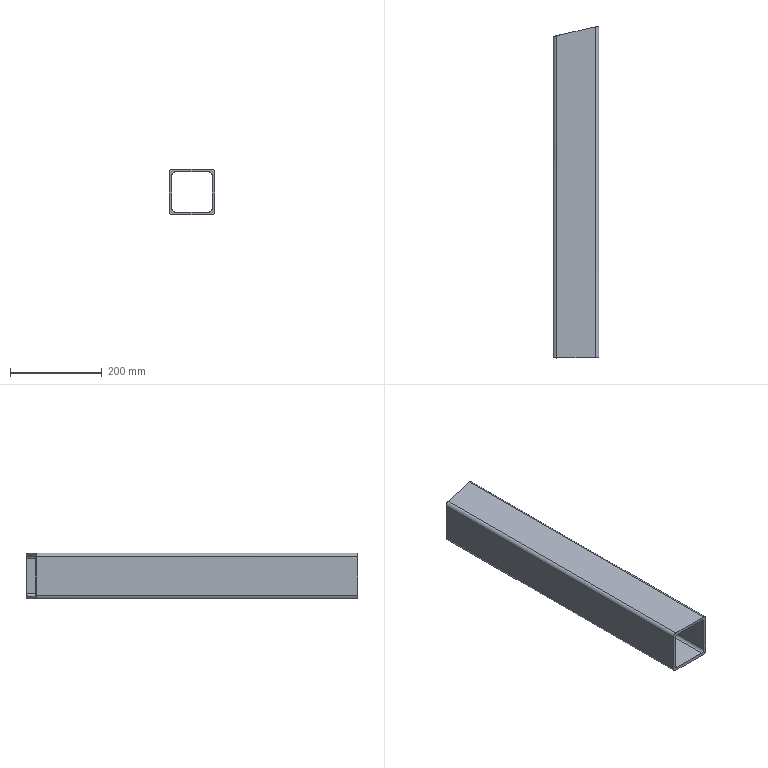Part | SolidWorks | features Extrusion 1, ICE 1 | 1 solid | 18 faces | box 100 x 723 x 100 mm | volume 1666387 mm3 | plane 10 | cylinder 8 | commonest cylinder face diameters 12.6 x4 15.75 x4
STEP:
#1=CARTESIAN_POINT('',(100.,-361.5,-90.6));
#2=VERTEX_POINT('',#1);
#3=CARTESIAN_POINT('',(92.125,-361.5,-98.475));
#4=VERTEX_POINT('',#3);
#5=CARTESIAN_POINT('',(92.125,-361.5,-90.6));
#6=DIRECTION('',(0.,1.,0.));
#7=DIRECTION('',(0.,0.,1.));
#8=AXIS2_PLACEMENT_3D('',#5,#6,#7);
#9=CIRCLE('',#8,7.875);
#10=EDGE_CURVE('',#2,#4,#9,.T.);
#11=ORIENTED_EDGE('',*,*,#10,.F.);
#12=CARTESIAN_POINT('',(100.,-361.5,-6.35));
#13=VERTEX_POINT('',#12);
#14=CARTESIAN_POINT('',(100.,-361.5,-90.6));
#15=DIRECTION('',(0.,0.,-1.));
#16=VECTOR('',#15,1000.);
#17=LINE('',#14,#16);
#18=EDGE_CURVE('',#13,#2,#17,.T.);
#19=ORIENTED_EDGE('',*,*,#18,.F.);
#20=CARTESIAN_POINT('',(92.125,-361.5,1.525));
#21=VERTEX_POINT('',#20);
#22=CARTESIAN_POINT('',(92.125,-361.5,-6.35));
#23=DIRECTION('',(0.,1.,0.));
#24=DIRECTION('',(0.,0.,1.));
#25=AXIS2_PLACEMENT_3D('',#22,#23,#24);
#26=CIRCLE('',#25,7.875);
#27=EDGE_CURVE('',#21,#13,#26,.T.);
#28=ORIENTED_EDGE('',*,*,#27,.F.);
#29=CARTESIAN_POINT('',(7.875,-361.5,1.525));
#30=VERTEX_POINT('',#29);
#31=CARTESIAN_POINT('',(7.875,-361.5,1.525));
#32=DIRECTION('',(1.,0.,0.));
#33=VECTOR('',#32,1000.);
#34=LINE('',#31,#33);
#35=EDGE_CURVE('',#30,#21,#34,.T.);
#36=ORIENTED_EDGE('',*,*,#35,.F.);
#37=CARTESIAN_POINT('',(0.,-361.5,-6.35));
#38=VERTEX_POINT('',#37);
#39=CARTESIAN_POINT('',(7.875,-361.5,-6.35));
#40=DIRECTION('',(0.,1.,0.));
#41=DIRECTION('',(0.,0.,1.));
#42=AXIS2_PLACEMENT_3D('',#39,#40,#41);
#43=CIRCLE('',#42,7.875);
#44=EDGE_CURVE('',#38,#30,#43,.T.);
#45=ORIENTED_EDGE('',*,*,#44,.F.);
#46=CARTESIAN_POINT('',(0.,-361.5,-90.6));
#47=VERTEX_POINT('',#46);
#48=CARTESIAN_POINT('',(0.,-361.5,-6.35));
#49=DIRECTION('',(0.,0.,1.));
#50=VECTOR('',#49,1000.);
#51=LINE('',#48,#50);
#52=EDGE_CURVE('',#47,#38,#51,.T.);
#53=ORIENTED_EDGE('',*,*,#52,.F.);
#54=CARTESIAN_POINT('',(7.875,-361.5,-98.475));
#55=VERTEX_POINT('',#54);
#56=CARTESIAN_POINT('',(7.875,-361.5,-90.6));
#57=DIRECTION('',(0.,1.,0.));
#58=DIRECTION('',(0.,0.,1.));
#59=AXIS2_PLACEMENT_3D('',#56,#57,#58);
#60=CIRCLE('',#59,7.875);
#61=EDGE_CURVE('',#55,#47,#60,.T.);
#62=ORIENTED_EDGE('',*,*,#61,.F.);
#63=CARTESIAN_POINT('',(92.125,-361.5,-98.475));
#64=DIRECTION('',(-1.,0.,0.));
#65=VECTOR('',#64,1000.);
#66=LINE('',#63,#65);
#67=EDGE_CURVE('',#4,#55,#66,.T.);
#68=ORIENTED_EDGE('',*,*,#67,.F.);
#69=EDGE_LOOP('',(#11,#19,#28,#36,#45,#53,#62,#68));
#70=FACE_OUTER_BOUND('',#69,.T.);
#71=CARTESIAN_POINT('',(12.6,-361.5,-92.175));
#72=VERTEX_POINT('',#71);
#73=CARTESIAN_POINT('',(6.3,-361.5,-85.875));
#74=VERTEX_POINT('',#73);
#75=CARTESIAN_POINT('',(12.6,-361.5,-85.875));
#76=DIRECTION('',(0.,1.,0.));
#77=DIRECTION('',(0.,0.,1.));
#78=AXIS2_PLACEMENT_3D('',#75,#76,#77);
#79=CIRCLE('',#78,6.3);
#80=EDGE_CURVE('',#72,#74,#79,.T.);
#81=ORIENTED_EDGE('',*,*,#80,.T.);
#82=CARTESIAN_POINT('',(6.3,-361.5,-11.075));
#83=VERTEX_POINT('',#82);
#84=CARTESIAN_POINT('',(6.3,-361.5,-11.075));
#85=DIRECTION('',(0.,0.,1.));
#86=VECTOR('',#85,1000.);
#87=LINE('',#84,#86);
#88=EDGE_CURVE('',#74,#83,#87,.T.);
#89=ORIENTED_EDGE('',*,*,#88,.T.);
#90=CARTESIAN_POINT('',(12.6,-361.5,-4.775));
#91=VERTEX_POINT('',#90);
#92=CARTESIAN_POINT('',(12.6,-361.5,-11.075));
#93=DIRECTION('',(0.,1.,0.));
#94=DIRECTION('',(0.,0.,1.));
#95=AXIS2_PLACEMENT_3D('',#92,#93,#94);
#96=CIRCLE('',#95,6.3);
#97=EDGE_CURVE('',#83,#91,#96,.T.);
#98=ORIENTED_EDGE('',*,*,#97,.T.);
#99=CARTESIAN_POINT('',(87.4,-361.5,-4.775));
#100=VERTEX_POINT('',#99);
#101=CARTESIAN_POINT('',(12.6,-361.5,-4.775));
#102=DIRECTION('',(1.,0.,0.));
#103=VECTOR('',#102,1000.);
#104=LINE('',#101,#103);
#105=EDGE_CURVE('',#91,#100,#104,.T.);
#106=ORIENTED_EDGE('',*,*,#105,.T.);
#107=CARTESIAN_POINT('',(93.7,-361.5,-11.075));
#108=VERTEX_POINT('',#107);
#109=CARTESIAN_POINT('',(87.4,-361.5,-11.075));
#110=DIRECTION('',(0.,1.,0.));
#111=DIRECTION('',(0.,0.,1.));
#112=AXIS2_PLACEMENT_3D('',#109,#110,#111);
#113=CIRCLE('',#112,6.3);
#114=EDGE_CURVE('',#100,#108,#113,.T.);
#115=ORIENTED_EDGE('',*,*,#114,.T.);
#116=CARTESIAN_POINT('',(93.7,-361.5,-85.875));
#117=VERTEX_POINT('',#116);
#118=CARTESIAN_POINT('',(93.7,-361.5,-85.875));
#119=DIRECTION('',(0.,0.,-1.));
#120=VECTOR('',#119,1000.);
#121=LINE('',#118,#120);
#122=EDGE_CURVE('',#108,#117,#121,.T.);
#123=ORIENTED_EDGE('',*,*,#122,.T.);
#124=CARTESIAN_POINT('',(87.4,-361.5,-92.175));
#125=VERTEX_POINT('',#124);
#126=CARTESIAN_POINT('',(87.4,-361.5,-85.875));
#127=DIRECTION('',(0.,1.,0.));
#128=DIRECTION('',(0.,0.,1.));
#129=AXIS2_PLACEMENT_3D('',#126,#127,#128);
#130=CIRCLE('',#129,6.3);
#131=EDGE_CURVE('',#117,#125,#130,.T.);
#132=ORIENTED_EDGE('',*,*,#131,.T.);
#133=CARTESIAN_POINT('',(87.4,-361.5,-92.175));
#134=DIRECTION('',(-1.,0.,0.));
#135=VECTOR('',#134,1000.);
#136=LINE('',#133,#135);
#137=EDGE_CURVE('',#125,#72,#136,.T.);
#138=ORIENTED_EDGE('',*,*,#137,.T.);
#139=EDGE_LOOP('',(#81,#89,#98,#106,#115,#123,#132,#138));
#140=FACE_BOUND('',#139,.T.);
#141=CARTESIAN_POINT('',(92.125,-361.5,-90.6));
#142=DIRECTION('',(0.,1.,0.));
#143=DIRECTION('',(0.,0.,1.));
#144=AXIS2_PLACEMENT_3D('',#141,#142,#143);
#145=PLANE('',#144);
#146=ADVANCED_FACE('',(#70,#140),#145,.F.);
#147=CARTESIAN_POINT('',(92.125,359.689,-98.475));
#148=VERTEX_POINT('',#147);
#149=CARTESIAN_POINT('',(92.125,361.5,-98.475));
#150=DIRECTION('',(0.,-1.,0.));
#151=VECTOR('',#150,1000.);
#152=LINE('',#149,#151);
#153=EDGE_CURVE('',#148,#4,#152,.T.);
#154=ORIENTED_EDGE('',*,*,#153,.F.);
#155=CARTESIAN_POINT('',(100.,361.5,-90.6));
#156=VERTEX_POINT('',#155);
#157=CARTESIAN_POINT('',(100.,361.5,-90.6));
#158=CARTESIAN_POINT('',(100.,361.5,-95.213));
#159=CARTESIAN_POINT('',(96.738,360.75,-98.475));
#160=CARTESIAN_POINT('',(92.125,359.689,-98.475));
#161=(BOUNDED_CURVE()B_SPLINE_CURVE(3,(#157,#158,#159,#160),.UNSPECIFIED.,.F.,.F.)B_SPLINE_CURVE_WITH_KNOTS((4,4),(3.142,4.712),.UNSPECIFIED.)CURVE()GEOMETRIC_REPRESENTATION_ITEM()RATIONAL_B_SPLINE_CURVE((1.,0.8047,0.8047,1.))REPRESENTATION_ITEM(''));
#162=EDGE_CURVE('',#156,#148,#161,.T.);
#163=ORIENTED_EDGE('',*,*,#162,.F.);
#164=CARTESIAN_POINT('',(100.,361.5,-90.6));
#165=DIRECTION('',(0.,-1.,0.));
#166=VECTOR('',#165,1000.);
#167=LINE('',#164,#166);
#168=EDGE_CURVE('',#156,#2,#167,.T.);
#169=ORIENTED_EDGE('',*,*,#168,.T.);
#170=ORIENTED_EDGE('',*,*,#10,.T.);
#171=EDGE_LOOP('',(#154,#163,#169,#170));
#172=FACE_OUTER_BOUND('',#171,.T.);
#173=CARTESIAN_POINT('',(92.125,361.5,-90.6));
#174=DIRECTION('',(0.,-1.,0.));
#175=DIRECTION('',(0.,0.,-1.));
#176=AXIS2_PLACEMENT_3D('',#173,#174,#175);
#177=CYLINDRICAL_SURFACE('',#176,7.875);
#178=ADVANCED_FACE('',(#172),#177,.T.);
#179=CARTESIAN_POINT('',(7.875,340.311,-98.475));
#180=VERTEX_POINT('',#179);
#181=CARTESIAN_POINT('',(7.875,361.5,-98.475));
#182=DIRECTION('',(0.,-1.,0.));
#183=VECTOR('',#182,1000.);
#184=LINE('',#181,#183);
#185=EDGE_CURVE('',#180,#55,#184,.T.);
#186=ORIENTED_EDGE('',*,*,#185,.F.);
#187=CARTESIAN_POINT('',(100.,361.5,-98.475));
#188=DIRECTION('',(-0.9746,-0.2241,0.));
#189=VECTOR('',#188,1000.);
#190=LINE('',#187,#189);
#191=EDGE_CURVE('',#148,#180,#190,.T.);
#192=ORIENTED_EDGE('',*,*,#191,.F.);
#193=ORIENTED_EDGE('',*,*,#153,.T.);
#194=ORIENTED_EDGE('',*,*,#67,.T.);
#195=EDGE_LOOP('',(#186,#192,#193,#194));
#196=FACE_OUTER_BOUND('',#195,.T.);
#197=CARTESIAN_POINT('',(92.125,361.5,-98.475));
#198=DIRECTION('',(0.,0.,1.));
#199=DIRECTION('',(1.,0.,0.));
#200=AXIS2_PLACEMENT_3D('',#197,#198,#199);
#201=PLANE('',#200);
#202=ADVANCED_FACE('',(#196),#201,.F.);
#203=CARTESIAN_POINT('',(0.,338.5,-90.6));
#204=VERTEX_POINT('',#203);
#205=CARTESIAN_POINT('',(0.,361.5,-90.6));
#206=DIRECTION('',(0.,-1.,0.));
#207=VECTOR('',#206,1000.);
#208=LINE('',#205,#207);
#209=EDGE_CURVE('',#204,#47,#208,.T.);
#210=ORIENTED_EDGE('',*,*,#209,.F.);
#211=CARTESIAN_POINT('',(7.875,340.311,-98.475));
#212=CARTESIAN_POINT('',(3.262,339.25,-98.475));
#213=CARTESIAN_POINT('',(0.,338.5,-95.213));
#214=CARTESIAN_POINT('',(0.,338.5,-90.6));
#215=(BOUNDED_CURVE()B_SPLINE_CURVE(3,(#211,#212,#213,#214),.UNSPECIFIED.,.F.,.T.)B_SPLINE_CURVE_WITH_KNOTS((4,4),(4.712,6.283),.UNSPECIFIED.)CURVE()GEOMETRIC_REPRESENTATION_ITEM()RATIONAL_B_SPLINE_CURVE((1.,0.8047,0.8047,1.))REPRESENTATION_ITEM(''));
#216=EDGE_CURVE('',#180,#204,#215,.T.);
#217=ORIENTED_EDGE('',*,*,#216,.F.);
#218=ORIENTED_EDGE('',*,*,#185,.T.);
#219=ORIENTED_EDGE('',*,*,#61,.T.);
#220=EDGE_LOOP('',(#210,#217,#218,#219));
#221=FACE_OUTER_BOUND('',#220,.T.);
#222=CARTESIAN_POINT('',(7.875,361.5,-90.6));
#223=DIRECTION('',(0.,-1.,0.));
#224=DIRECTION('',(0.,0.,-1.));
#225=AXIS2_PLACEMENT_3D('',#222,#223,#224);
#226=CYLINDRICAL_SURFACE('',#225,7.875);
#227=ADVANCED_FACE('',(#221),#226,.T.);
#228=CARTESIAN_POINT('',(0.,338.5,-6.35));
#229=VERTEX_POINT('',#228);
#230=CARTESIAN_POINT('',(0.,361.5,-6.35));
#231=DIRECTION('',(0.,-1.,0.));
#232=VECTOR('',#231,1000.);
#233=LINE('',#230,#232);
#234=EDGE_CURVE('',#229,#38,#233,.T.);
#235=ORIENTED_EDGE('',*,*,#234,.F.);
#236=CARTESIAN_POINT('',(0.,338.5,-98.476));
#237=DIRECTION('',(0.,0.,1.));
#238=VECTOR('',#237,1000.);
#239=LINE('',#236,#238);
#240=EDGE_CURVE('',#204,#229,#239,.T.);
#241=ORIENTED_EDGE('',*,*,#240,.F.);
#242=ORIENTED_EDGE('',*,*,#209,.T.);
#243=ORIENTED_EDGE('',*,*,#52,.T.);
#244=EDGE_LOOP('',(#235,#241,#242,#243));
#245=FACE_OUTER_BOUND('',#244,.T.);
#246=CARTESIAN_POINT('',(0.,361.5,-6.35));
#247=DIRECTION('',(1.,0.,0.));
#248=DIRECTION('',(0.,0.,-1.));
#249=AXIS2_PLACEMENT_3D('',#246,#247,#248);
#250=PLANE('',#249);
#251=ADVANCED_FACE('',(#245),#250,.F.);
#252=CARTESIAN_POINT('',(7.875,340.311,1.525));
#253=VERTEX_POINT('',#252);
#254=CARTESIAN_POINT('',(7.875,361.5,1.525));
#255=DIRECTION('',(0.,-1.,0.));
#256=VECTOR('',#255,1000.);
#257=LINE('',#254,#256);
#258=EDGE_CURVE('',#253,#30,#257,.T.);
#259=ORIENTED_EDGE('',*,*,#258,.F.);
#260=CARTESIAN_POINT('',(0.,338.5,-6.35));
#261=CARTESIAN_POINT('',(0.,338.5,-1.737));
#262=CARTESIAN_POINT('',(3.262,339.25,1.525));
#263=CARTESIAN_POINT('',(7.875,340.311,1.525));
#264=(BOUNDED_CURVE()B_SPLINE_CURVE(3,(#260,#261,#262,#263),.UNSPECIFIED.,.F.,.T.)B_SPLINE_CURVE_WITH_KNOTS((4,4),(0.,1.571),.UNSPECIFIED.)CURVE()GEOMETRIC_REPRESENTATION_ITEM()RATIONAL_B_SPLINE_CURVE((1.,0.8047,0.8047,1.))REPRESENTATION_ITEM(''));
#265=EDGE_CURVE('',#229,#253,#264,.T.);
#266=ORIENTED_EDGE('',*,*,#265,.F.);
#267=ORIENTED_EDGE('',*,*,#234,.T.);
#268=ORIENTED_EDGE('',*,*,#44,.T.);
#269=EDGE_LOOP('',(#259,#266,#267,#268));
#270=FACE_OUTER_BOUND('',#269,.T.);
#271=CARTESIAN_POINT('',(7.875,361.5,-6.35));
#272=DIRECTION('',(0.,-1.,0.));
#273=DIRECTION('',(0.,0.,-1.));
#274=AXIS2_PLACEMENT_3D('',#271,#272,#273);
#275=CYLINDRICAL_SURFACE('',#274,7.875);
#276=ADVANCED_FACE('',(#270),#275,.T.);
#277=CARTESIAN_POINT('',(92.125,359.689,1.525));
#278=VERTEX_POINT('',#277);
#279=CARTESIAN_POINT('',(92.125,361.5,1.525));
#280=DIRECTION('',(0.,-1.,0.));
#281=VECTOR('',#280,1000.);
#282=LINE('',#279,#281);
#283=EDGE_CURVE('',#278,#21,#282,.T.);
#284=ORIENTED_EDGE('',*,*,#283,.F.);
#285=CARTESIAN_POINT('',(100.,361.5,1.525));
#286=DIRECTION('',(0.9746,0.2241,0.));
#287=VECTOR('',#286,1000.);
#288=LINE('',#285,#287);
#289=EDGE_CURVE('',#253,#278,#288,.T.);
#290=ORIENTED_EDGE('',*,*,#289,.F.);
#291=ORIENTED_EDGE('',*,*,#258,.T.);
#292=ORIENTED_EDGE('',*,*,#35,.T.);
#293=EDGE_LOOP('',(#284,#290,#291,#292));
#294=FACE_OUTER_BOUND('',#293,.T.);
#295=CARTESIAN_POINT('',(7.875,361.5,1.525));
#296=DIRECTION('',(0.,0.,-1.));
#297=DIRECTION('',(-1.,0.,0.));
#298=AXIS2_PLACEMENT_3D('',#295,#296,#297);
#299=PLANE('',#298);
#300=ADVANCED_FACE('',(#294),#299,.F.);
#301=CARTESIAN_POINT('',(100.,361.5,-6.35));
#302=VERTEX_POINT('',#301);
#303=CARTESIAN_POINT('',(100.,361.5,-6.35));
#304=DIRECTION('',(0.,-1.,0.));
#305=VECTOR('',#304,1000.);
#306=LINE('',#303,#305);
#307=EDGE_CURVE('',#302,#13,#306,.T.);
#308=ORIENTED_EDGE('',*,*,#307,.F.);
#309=CARTESIAN_POINT('',(92.125,359.689,1.525));
#310=CARTESIAN_POINT('',(96.738,360.75,1.525));
#311=CARTESIAN_POINT('',(100.,361.5,-1.737));
#312=CARTESIAN_POINT('',(100.,361.5,-6.35));
#313=(BOUNDED_CURVE()B_SPLINE_CURVE(3,(#309,#310,#311,#312),.UNSPECIFIED.,.F.,.F.)B_SPLINE_CURVE_WITH_KNOTS((4,4),(1.571,3.142),.UNSPECIFIED.)CURVE()GEOMETRIC_REPRESENTATION_ITEM()RATIONAL_B_SPLINE_CURVE((1.,0.8047,0.8047,1.))REPRESENTATION_ITEM(''));
#314=EDGE_CURVE('',#278,#302,#313,.T.);
#315=ORIENTED_EDGE('',*,*,#314,.F.);
#316=ORIENTED_EDGE('',*,*,#283,.T.);
#317=ORIENTED_EDGE('',*,*,#27,.T.);
#318=EDGE_LOOP('',(#308,#315,#316,#317));
#319=FACE_OUTER_BOUND('',#318,.T.);
#320=CARTESIAN_POINT('',(92.125,361.5,-6.35));
#321=DIRECTION('',(0.,-1.,0.));
#322=DIRECTION('',(0.,0.,-1.));
#323=AXIS2_PLACEMENT_3D('',#320,#321,#322);
#324=CYLINDRICAL_SURFACE('',#323,7.875);
#325=ADVANCED_FACE('',(#319),#324,.T.);
#326=ORIENTED_EDGE('',*,*,#18,.T.);
#327=ORIENTED_EDGE('',*,*,#168,.F.);
#328=CARTESIAN_POINT('',(100.,361.5,-90.6));
#329=DIRECTION('',(0.,0.,-1.));
#330=VECTOR('',#329,1000.);
#331=LINE('',#328,#330);
#332=EDGE_CURVE('',#302,#156,#331,.T.);
#333=ORIENTED_EDGE('',*,*,#332,.F.);
#334=ORIENTED_EDGE('',*,*,#307,.T.);
#335=EDGE_LOOP('',(#326,#327,#333,#334));
#336=FACE_OUTER_BOUND('',#335,.T.);
#337=CARTESIAN_POINT('',(100.,361.5,-90.6));
#338=DIRECTION('',(-1.,0.,0.));
#339=DIRECTION('',(0.,0.,1.));
#340=AXIS2_PLACEMENT_3D('',#337,#338,#339);
#341=PLANE('',#340);
#342=ADVANCED_FACE('',(#336),#341,.F.);
#343=CARTESIAN_POINT('',(12.6,341.398,-92.175));
#344=VERTEX_POINT('',#343);
#345=CARTESIAN_POINT('',(6.3,339.949,-85.875));
#346=VERTEX_POINT('',#345);
#347=CARTESIAN_POINT('',(12.6,341.398,-92.175));
#348=CARTESIAN_POINT('',(8.91,340.549,-92.175));
#349=CARTESIAN_POINT('',(6.3,339.949,-89.565));
#350=CARTESIAN_POINT('',(6.3,339.949,-85.875));
#351=(BOUNDED_CURVE()B_SPLINE_CURVE(3,(#347,#348,#349,#350),.UNSPECIFIED.,.F.,.F.)B_SPLINE_CURVE_WITH_KNOTS((4,4),(4.712,6.283),.UNSPECIFIED.)CURVE()GEOMETRIC_REPRESENTATION_ITEM()RATIONAL_B_SPLINE_CURVE((1.,0.8047,0.8047,1.))REPRESENTATION_ITEM(''));
#352=EDGE_CURVE('',#344,#346,#351,.T.);
#353=ORIENTED_EDGE('',*,*,#352,.T.);
#354=CARTESIAN_POINT('',(6.3,361.5,-85.875));
#355=DIRECTION('',(0.,-1.,0.));
#356=VECTOR('',#355,1000.);
#357=LINE('',#354,#356);
#358=EDGE_CURVE('',#346,#74,#357,.T.);
#359=ORIENTED_EDGE('',*,*,#358,.T.);
#360=ORIENTED_EDGE('',*,*,#80,.F.);
#361=CARTESIAN_POINT('',(12.6,361.5,-92.175));
#362=DIRECTION('',(0.,-1.,0.));
#363=VECTOR('',#362,1000.);
#364=LINE('',#361,#363);
#365=EDGE_CURVE('',#344,#72,#364,.T.);
#366=ORIENTED_EDGE('',*,*,#365,.F.);
#367=EDGE_LOOP('',(#353,#359,#360,#366));
#368=FACE_OUTER_BOUND('',#367,.T.);
#369=CARTESIAN_POINT('',(12.6,361.5,-85.875));
#370=DIRECTION('',(0.,-1.,0.));
#371=DIRECTION('',(0.,0.,-1.));
#372=AXIS2_PLACEMENT_3D('',#369,#370,#371);
#373=CYLINDRICAL_SURFACE('',#372,6.3);
#374=ADVANCED_FACE('',(#368),#373,.F.);
#375=CARTESIAN_POINT('',(6.3,339.949,-11.075));
#376=VERTEX_POINT('',#375);
#377=CARTESIAN_POINT('',(6.3,339.949,-98.476));
#378=DIRECTION('',(0.,0.,1.));
#379=VECTOR('',#378,1000.);
#380=LINE('',#377,#379);
#381=EDGE_CURVE('',#346,#376,#380,.T.);
#382=ORIENTED_EDGE('',*,*,#381,.T.);
#383=CARTESIAN_POINT('',(6.3,361.5,-11.075));
#384=DIRECTION('',(0.,-1.,0.));
#385=VECTOR('',#384,1000.);
#386=LINE('',#383,#385);
#387=EDGE_CURVE('',#376,#83,#386,.T.);
#388=ORIENTED_EDGE('',*,*,#387,.T.);
#389=ORIENTED_EDGE('',*,*,#88,.F.);
#390=ORIENTED_EDGE('',*,*,#358,.F.);
#391=EDGE_LOOP('',(#382,#388,#389,#390));
#392=FACE_OUTER_BOUND('',#391,.T.);
#393=CARTESIAN_POINT('',(6.3,361.5,-11.075));
#394=DIRECTION('',(1.,0.,0.));
#395=DIRECTION('',(0.,0.,-1.));
#396=AXIS2_PLACEMENT_3D('',#393,#394,#395);
#397=PLANE('',#396);
#398=ADVANCED_FACE('',(#392),#397,.T.);
#399=CARTESIAN_POINT('',(12.6,341.398,-4.775));
#400=VERTEX_POINT('',#399);
#401=CARTESIAN_POINT('',(6.3,339.949,-11.075));
#402=CARTESIAN_POINT('',(6.3,339.949,-7.385));
#403=CARTESIAN_POINT('',(8.91,340.549,-4.775));
#404=CARTESIAN_POINT('',(12.6,341.398,-4.775));
#405=(BOUNDED_CURVE()B_SPLINE_CURVE(3,(#401,#402,#403,#404),.UNSPECIFIED.,.F.,.T.)B_SPLINE_CURVE_WITH_KNOTS((4,4),(0.,1.571),.UNSPECIFIED.)CURVE()GEOMETRIC_REPRESENTATION_ITEM()RATIONAL_B_SPLINE_CURVE((1.,0.8047,0.8047,1.))REPRESENTATION_ITEM(''));
#406=EDGE_CURVE('',#376,#400,#405,.T.);
#407=ORIENTED_EDGE('',*,*,#406,.T.);
#408=CARTESIAN_POINT('',(12.6,361.5,-4.775));
#409=DIRECTION('',(0.,-1.,0.));
#410=VECTOR('',#409,1000.);
#411=LINE('',#408,#410);
#412=EDGE_CURVE('',#400,#91,#411,.T.);
#413=ORIENTED_EDGE('',*,*,#412,.T.);
#414=ORIENTED_EDGE('',*,*,#97,.F.);
#415=ORIENTED_EDGE('',*,*,#387,.F.);
#416=EDGE_LOOP('',(#407,#413,#414,#415));
#417=FACE_OUTER_BOUND('',#416,.T.);
#418=CARTESIAN_POINT('',(12.6,361.5,-11.075));
#419=DIRECTION('',(0.,-1.,0.));
#420=DIRECTION('',(0.,0.,-1.));
#421=AXIS2_PLACEMENT_3D('',#418,#419,#420);
#422=CYLINDRICAL_SURFACE('',#421,6.3);
#423=ADVANCED_FACE('',(#417),#422,.F.);
#424=CARTESIAN_POINT('',(87.4,358.602,-4.775));
#425=VERTEX_POINT('',#424);
#426=CARTESIAN_POINT('',(100.,361.5,-4.775));
#427=DIRECTION('',(0.9746,0.2241,0.));
#428=VECTOR('',#427,1000.);
#429=LINE('',#426,#428);
#430=EDGE_CURVE('',#400,#425,#429,.T.);
#431=ORIENTED_EDGE('',*,*,#430,.T.);
#432=CARTESIAN_POINT('',(87.4,361.5,-4.775));
#433=DIRECTION('',(0.,-1.,0.));
#434=VECTOR('',#433,1000.);
#435=LINE('',#432,#434);
#436=EDGE_CURVE('',#425,#100,#435,.T.);
#437=ORIENTED_EDGE('',*,*,#436,.T.);
#438=ORIENTED_EDGE('',*,*,#105,.F.);
#439=ORIENTED_EDGE('',*,*,#412,.F.);
#440=EDGE_LOOP('',(#431,#437,#438,#439));
#441=FACE_OUTER_BOUND('',#440,.T.);
#442=CARTESIAN_POINT('',(12.6,361.5,-4.775));
#443=DIRECTION('',(0.,0.,-1.));
#444=DIRECTION('',(-1.,0.,0.));
#445=AXIS2_PLACEMENT_3D('',#442,#443,#444);
#446=PLANE('',#445);
#447=ADVANCED_FACE('',(#441),#446,.T.);
#448=CARTESIAN_POINT('',(93.7,360.051,-11.075));
#449=VERTEX_POINT('',#448);
#450=CARTESIAN_POINT('',(87.4,358.602,-4.775));
#451=CARTESIAN_POINT('',(91.09,359.451,-4.775));
#452=CARTESIAN_POINT('',(93.7,360.051,-7.385));
#453=CARTESIAN_POINT('',(93.7,360.051,-11.075));
#454=(BOUNDED_CURVE()B_SPLINE_CURVE(3,(#450,#451,#452,#453),.UNSPECIFIED.,.F.,.T.)B_SPLINE_CURVE_WITH_KNOTS((4,4),(1.571,3.142),.UNSPECIFIED.)CURVE()GEOMETRIC_REPRESENTATION_ITEM()RATIONAL_B_SPLINE_CURVE((1.,0.8047,0.8047,1.))REPRESENTATION_ITEM(''));
#455=EDGE_CURVE('',#425,#449,#454,.T.);
#456=ORIENTED_EDGE('',*,*,#455,.T.);
#457=CARTESIAN_POINT('',(93.7,361.5,-11.075));
#458=DIRECTION('',(0.,-1.,0.));
#459=VECTOR('',#458,1000.);
#460=LINE('',#457,#459);
#461=EDGE_CURVE('',#449,#108,#460,.T.);
#462=ORIENTED_EDGE('',*,*,#461,.T.);
#463=ORIENTED_EDGE('',*,*,#114,.F.);
#464=ORIENTED_EDGE('',*,*,#436,.F.);
#465=EDGE_LOOP('',(#456,#462,#463,#464));
#466=FACE_OUTER_BOUND('',#465,.T.);
#467=CARTESIAN_POINT('',(87.4,361.5,-11.075));
#468=DIRECTION('',(0.,-1.,0.));
#469=DIRECTION('',(0.,0.,-1.));
#470=AXIS2_PLACEMENT_3D('',#467,#468,#469);
#471=CYLINDRICAL_SURFACE('',#470,6.3);
#472=ADVANCED_FACE('',(#466),#471,.F.);
#473=CARTESIAN_POINT('',(93.7,360.051,-85.875));
#474=VERTEX_POINT('',#473);
#475=CARTESIAN_POINT('',(93.7,360.051,-98.476));
#476=DIRECTION('',(0.,0.,-1.));
#477=VECTOR('',#476,1000.);
#478=LINE('',#475,#477);
#479=EDGE_CURVE('',#449,#474,#478,.T.);
#480=ORIENTED_EDGE('',*,*,#479,.T.);
#481=CARTESIAN_POINT('',(93.7,361.5,-85.875));
#482=DIRECTION('',(0.,-1.,0.));
#483=VECTOR('',#482,1000.);
#484=LINE('',#481,#483);
#485=EDGE_CURVE('',#474,#117,#484,.T.);
#486=ORIENTED_EDGE('',*,*,#485,.T.);
#487=ORIENTED_EDGE('',*,*,#122,.F.);
#488=ORIENTED_EDGE('',*,*,#461,.F.);
#489=EDGE_LOOP('',(#480,#486,#487,#488));
#490=FACE_OUTER_BOUND('',#489,.T.);
#491=CARTESIAN_POINT('',(93.7,361.5,-85.875));
#492=DIRECTION('',(-1.,0.,0.));
#493=DIRECTION('',(0.,0.,1.));
#494=AXIS2_PLACEMENT_3D('',#491,#492,#493);
#495=PLANE('',#494);
#496=ADVANCED_FACE('',(#490),#495,.T.);
#497=CARTESIAN_POINT('',(87.4,358.602,-92.175));
#498=VERTEX_POINT('',#497);
#499=CARTESIAN_POINT('',(93.7,360.051,-85.875));
#500=CARTESIAN_POINT('',(93.7,360.051,-89.565));
#501=CARTESIAN_POINT('',(91.09,359.451,-92.175));
#502=CARTESIAN_POINT('',(87.4,358.602,-92.175));
#503=(BOUNDED_CURVE()B_SPLINE_CURVE(3,(#499,#500,#501,#502),.UNSPECIFIED.,.F.,.T.)B_SPLINE_CURVE_WITH_KNOTS((4,4),(3.142,4.712),.UNSPECIFIED.)CURVE()GEOMETRIC_REPRESENTATION_ITEM()RATIONAL_B_SPLINE_CURVE((1.,0.8047,0.8047,1.))REPRESENTATION_ITEM(''));
#504=EDGE_CURVE('',#474,#498,#503,.T.);
#505=ORIENTED_EDGE('',*,*,#504,.T.);
#506=CARTESIAN_POINT('',(87.4,361.5,-92.175));
#507=DIRECTION('',(0.,-1.,0.));
#508=VECTOR('',#507,1000.);
#509=LINE('',#506,#508);
#510=EDGE_CURVE('',#498,#125,#509,.T.);
#511=ORIENTED_EDGE('',*,*,#510,.T.);
#512=ORIENTED_EDGE('',*,*,#131,.F.);
#513=ORIENTED_EDGE('',*,*,#485,.F.);
#514=EDGE_LOOP('',(#505,#511,#512,#513));
#515=FACE_OUTER_BOUND('',#514,.T.);
#516=CARTESIAN_POINT('',(87.4,361.5,-85.875));
#517=DIRECTION('',(0.,-1.,0.));
#518=DIRECTION('',(0.,0.,-1.));
#519=AXIS2_PLACEMENT_3D('',#516,#517,#518);
#520=CYLINDRICAL_SURFACE('',#519,6.3);
#521=ADVANCED_FACE('',(#515),#520,.F.);
#522=CARTESIAN_POINT('',(100.,361.5,-92.175));
#523=DIRECTION('',(-0.9746,-0.2241,0.));
#524=VECTOR('',#523,1000.);
#525=LINE('',#522,#524);
#526=EDGE_CURVE('',#498,#344,#525,.T.);
#527=ORIENTED_EDGE('',*,*,#526,.T.);
#528=ORIENTED_EDGE('',*,*,#365,.T.);
#529=ORIENTED_EDGE('',*,*,#137,.F.);
#530=ORIENTED_EDGE('',*,*,#510,.F.);
#531=EDGE_LOOP('',(#527,#528,#529,#530));
#532=FACE_OUTER_BOUND('',#531,.T.);
#533=CARTESIAN_POINT('',(87.4,361.5,-92.175));
#534=DIRECTION('',(0.,0.,1.));
#535=DIRECTION('',(1.,0.,0.));
#536=AXIS2_PLACEMENT_3D('',#533,#534,#535);
#537=PLANE('',#536);
#538=ADVANCED_FACE('',(#532),#537,.T.);
#539=ORIENTED_EDGE('',*,*,#526,.F.);
#540=ORIENTED_EDGE('',*,*,#504,.F.);
#541=ORIENTED_EDGE('',*,*,#479,.F.);
#542=ORIENTED_EDGE('',*,*,#455,.F.);
#543=ORIENTED_EDGE('',*,*,#430,.F.);
#544=ORIENTED_EDGE('',*,*,#406,.F.);
#545=ORIENTED_EDGE('',*,*,#381,.F.);
#546=ORIENTED_EDGE('',*,*,#352,.F.);
#547=EDGE_LOOP('',(#539,#540,#541,#542,#543,#544,#545,#546));
#548=FACE_BOUND('',#547,.T.);
#549=ORIENTED_EDGE('',*,*,#162,.T.);
#550=ORIENTED_EDGE('',*,*,#191,.T.);
#551=ORIENTED_EDGE('',*,*,#216,.T.);
#552=ORIENTED_EDGE('',*,*,#240,.T.);
#553=ORIENTED_EDGE('',*,*,#265,.T.);
#554=ORIENTED_EDGE('',*,*,#289,.T.);
#555=ORIENTED_EDGE('',*,*,#314,.T.);
#556=ORIENTED_EDGE('',*,*,#332,.T.);
#557=EDGE_LOOP('',(#549,#550,#551,#552,#553,#554,#555,#556));
#558=FACE_OUTER_BOUND('',#557,.T.);
#559=CARTESIAN_POINT('',(100.,361.5,-98.476));
#560=DIRECTION('',(0.2241,-0.9746,0.));
#561=DIRECTION('',(0.9746,0.2241,0.));
#562=AXIS2_PLACEMENT_3D('',#559,#560,#561);
#563=PLANE('',#562);
#564=ADVANCED_FACE('',(#548,#558),#563,.F.);
#565=CLOSED_SHELL('',(#146,#178,#202,#227,#251,#276,#300,#325,#342,#374,#398,#423,#447,#472,#496,#521,#538,#564));
#566=MANIFOLD_SOLID_BREP('',#565);
#567=CARTESIAN_POINT('',(0.,0.,0.));
#568=DIRECTION('',(0.,0.,1.));
#569=DIRECTION('',(1.,0.,0.));
#570=AXIS2_PLACEMENT_3D('',#567,#568,#569);
#571=(LENGTH_UNIT()NAMED_UNIT(*)SI_UNIT(.MILLI.,.METRE.));
#572=UNCERTAINTY_MEASURE_WITH_UNIT(LENGTH_MEASURE(0.00001),#571,'','');
#573=(NAMED_UNIT(*)PLANE_ANGLE_UNIT()SI_UNIT($,.RADIAN.));
#574=(NAMED_UNIT(*)SI_UNIT($,.STERADIAN.)SOLID_ANGLE_UNIT());
#575=(GEOMETRIC_REPRESENTATION_CONTEXT(3)GLOBAL_UNCERTAINTY_ASSIGNED_CONTEXT((#572))GLOBAL_UNIT_ASSIGNED_CONTEXT((#571,#573,#574))REPRESENTATION_CONTEXT('',''));
#576=ADVANCED_BREP_SHAPE_REPRESENTATION('',(#566,#570),#575);